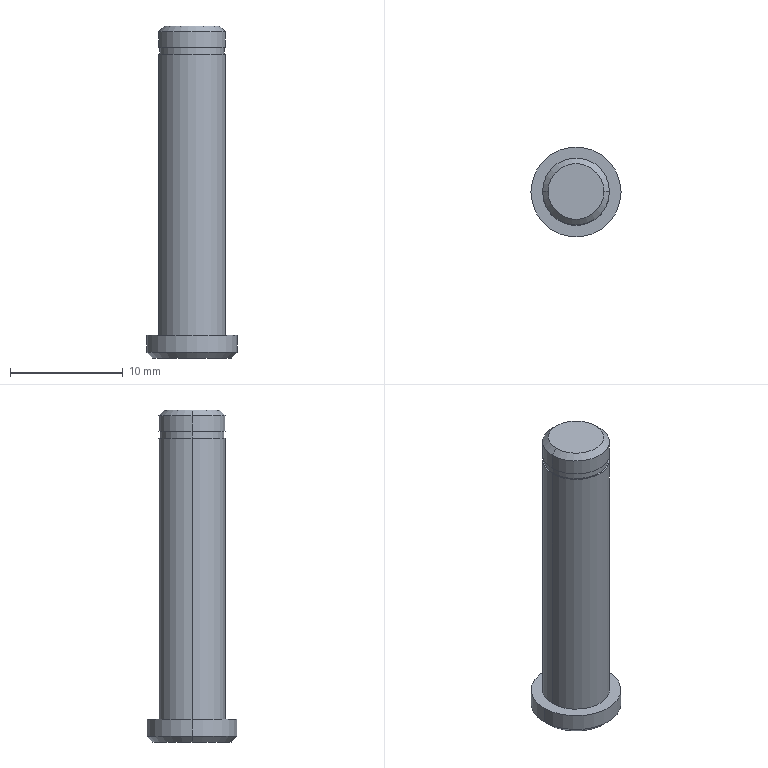Part | SolidWorks | features ICE 3, Chamfer 1, Extrusion 1 | 1 solid | 17 faces | box 8 x 8 x 29.5 mm | volume 858.581 mm3 | cylinder 8 | plane 5 | cone 4 | commonest cylinder face diameters 5.95 x4 5.7 x2 8 x2
STEP:
#1=CARTESIAN_POINT('',(2.475,0.,29.5));
#2=VERTEX_POINT('',#1);
#3=CARTESIAN_POINT('',(-2.475,0.,29.5));
#4=VERTEX_POINT('',#3);
#5=CARTESIAN_POINT('',(0.,0.,29.5));
#6=DIRECTION('',(0.,0.,1.));
#7=DIRECTION('',(1.,0.,0.));
#8=AXIS2_PLACEMENT_3D('',#5,#6,#7);
#9=CIRCLE('',#8,2.475);
#10=EDGE_CURVE('',#2,#4,#9,.T.);
#11=ORIENTED_EDGE('',*,*,#10,.F.);
#12=CARTESIAN_POINT('',(2.975,0.,29.));
#13=VERTEX_POINT('',#12);
#14=CARTESIAN_POINT('',(2.475,0.,29.5));
#15=DIRECTION('',(0.7071,0.,-0.7071));
#16=VECTOR('',#15,1000.);
#17=LINE('',#14,#16);
#18=EDGE_CURVE('',#2,#13,#17,.T.);
#19=ORIENTED_EDGE('',*,*,#18,.T.);
#20=CARTESIAN_POINT('',(-2.975,0.,29.));
#21=VERTEX_POINT('',#20);
#22=CARTESIAN_POINT('',(0.,0.,29.));
#23=DIRECTION('',(0.,0.,-1.));
#24=DIRECTION('',(1.,0.,0.));
#25=AXIS2_PLACEMENT_3D('',#22,#23,#24);
#26=CIRCLE('',#25,2.975);
#27=EDGE_CURVE('',#21,#13,#26,.T.);
#28=ORIENTED_EDGE('',*,*,#27,.F.);
#29=CARTESIAN_POINT('',(-2.475,0.,29.5));
#30=DIRECTION('',(-0.7071,0.,-0.7071));
#31=VECTOR('',#30,1000.);
#32=LINE('',#29,#31);
#33=EDGE_CURVE('',#4,#21,#32,.T.);
#34=ORIENTED_EDGE('',*,*,#33,.F.);
#35=EDGE_LOOP('',(#11,#19,#28,#34));
#36=FACE_OUTER_BOUND('',#35,.T.);
#37=CARTESIAN_POINT('',(0.,0.,29.5));
#38=DIRECTION('',(0.,0.,-1.));
#39=DIRECTION('',(-1.,0.,0.));
#40=AXIS2_PLACEMENT_3D('',#37,#38,#39);
#41=CONICAL_SURFACE('',#40,2.475,0.7854);
#42=ADVANCED_FACE('',(#36),#41,.T.);
#43=CARTESIAN_POINT('',(-3.5,0.,0.));
#44=VERTEX_POINT('',#43);
#45=CARTESIAN_POINT('',(3.5,0.,0.));
#46=VERTEX_POINT('',#45);
#47=CARTESIAN_POINT('',(0.,0.,0.));
#48=DIRECTION('',(0.,0.,-1.));
#49=DIRECTION('',(1.,0.,0.));
#50=AXIS2_PLACEMENT_3D('',#47,#48,#49);
#51=CIRCLE('',#50,3.5);
#52=EDGE_CURVE('',#44,#46,#51,.T.);
#53=ORIENTED_EDGE('',*,*,#52,.F.);
#54=CARTESIAN_POINT('',(-4.,0.,0.5));
#55=VERTEX_POINT('',#54);
#56=CARTESIAN_POINT('',(-4.,0.,0.5));
#57=DIRECTION('',(-0.7071,0.,0.7071));
#58=VECTOR('',#57,1000.);
#59=LINE('',#56,#58);
#60=EDGE_CURVE('',#44,#55,#59,.T.);
#61=ORIENTED_EDGE('',*,*,#60,.T.);
#62=CARTESIAN_POINT('',(4.,0.,0.5));
#63=VERTEX_POINT('',#62);
#64=CARTESIAN_POINT('',(0.,0.,0.5));
#65=DIRECTION('',(0.,0.,1.));
#66=DIRECTION('',(1.,0.,0.));
#67=AXIS2_PLACEMENT_3D('',#64,#65,#66);
#68=CIRCLE('',#67,4.);
#69=EDGE_CURVE('',#63,#55,#68,.T.);
#70=ORIENTED_EDGE('',*,*,#69,.F.);
#71=CARTESIAN_POINT('',(4.,0.,0.5));
#72=DIRECTION('',(0.7071,0.,0.7071));
#73=VECTOR('',#72,1000.);
#74=LINE('',#71,#73);
#75=EDGE_CURVE('',#46,#63,#74,.T.);
#76=ORIENTED_EDGE('',*,*,#75,.F.);
#77=EDGE_LOOP('',(#53,#61,#70,#76));
#78=FACE_OUTER_BOUND('',#77,.T.);
#79=CARTESIAN_POINT('',(0.,0.,0.5));
#80=DIRECTION('',(0.,0.,1.));
#81=DIRECTION('',(1.,0.,0.));
#82=AXIS2_PLACEMENT_3D('',#79,#80,#81);
#83=CONICAL_SURFACE('',#82,4.,0.7854);
#84=ADVANCED_FACE('',(#78),#83,.T.);
#85=ORIENTED_EDGE('',*,*,#27,.T.);
#86=CARTESIAN_POINT('',(2.975,0.,27.6));
#87=VERTEX_POINT('',#86);
#88=CARTESIAN_POINT('',(2.975,0.,29.5));
#89=DIRECTION('',(0.,0.,-1.));
#90=VECTOR('',#89,1000.);
#91=LINE('',#88,#90);
#92=EDGE_CURVE('',#13,#87,#91,.T.);
#93=ORIENTED_EDGE('',*,*,#92,.T.);
#94=CARTESIAN_POINT('',(-2.975,0.,27.6));
#95=VERTEX_POINT('',#94);
#96=CARTESIAN_POINT('',(0.,0.,27.6));
#97=DIRECTION('',(0.,0.,1.));
#98=DIRECTION('',(1.,0.,0.));
#99=AXIS2_PLACEMENT_3D('',#96,#97,#98);
#100=CIRCLE('',#99,2.975);
#101=EDGE_CURVE('',#87,#95,#100,.T.);
#102=ORIENTED_EDGE('',*,*,#101,.T.);
#103=CARTESIAN_POINT('',(-2.975,0.,29.5));
#104=DIRECTION('',(0.,0.,-1.));
#105=VECTOR('',#104,1000.);
#106=LINE('',#103,#105);
#107=EDGE_CURVE('',#21,#95,#106,.T.);
#108=ORIENTED_EDGE('',*,*,#107,.F.);
#109=EDGE_LOOP('',(#85,#93,#102,#108));
#110=FACE_OUTER_BOUND('',#109,.T.);
#111=CARTESIAN_POINT('',(0.,0.,29.5));
#112=DIRECTION('',(0.,0.,-1.));
#113=DIRECTION('',(-1.,0.,0.));
#114=AXIS2_PLACEMENT_3D('',#111,#112,#113);
#115=CYLINDRICAL_SURFACE('',#114,2.975);
#116=ADVANCED_FACE('',(#110),#115,.T.);
#117=CARTESIAN_POINT('',(2.85,0.,27.6));
#118=VERTEX_POINT('',#117);
#119=CARTESIAN_POINT('',(-2.85,0.,27.6));
#120=VERTEX_POINT('',#119);
#121=CARTESIAN_POINT('',(0.,0.,27.6));
#122=DIRECTION('',(0.,0.,1.));
#123=DIRECTION('',(1.,0.,0.));
#124=AXIS2_PLACEMENT_3D('',#121,#122,#123);
#125=CIRCLE('',#124,2.85);
#126=EDGE_CURVE('',#118,#120,#125,.T.);
#127=ORIENTED_EDGE('',*,*,#126,.F.);
#128=CARTESIAN_POINT('',(2.85,0.,27.));
#129=VERTEX_POINT('',#128);
#130=CARTESIAN_POINT('',(2.85,0.,27.6));
#131=DIRECTION('',(0.,0.,-1.));
#132=VECTOR('',#131,1000.);
#133=LINE('',#130,#132);
#134=EDGE_CURVE('',#118,#129,#133,.T.);
#135=ORIENTED_EDGE('',*,*,#134,.T.);
#136=CARTESIAN_POINT('',(-2.85,0.,27.));
#137=VERTEX_POINT('',#136);
#138=CARTESIAN_POINT('',(0.,0.,27.));
#139=DIRECTION('',(0.,0.,1.));
#140=DIRECTION('',(1.,0.,0.));
#141=AXIS2_PLACEMENT_3D('',#138,#139,#140);
#142=CIRCLE('',#141,2.85);
#143=EDGE_CURVE('',#129,#137,#142,.T.);
#144=ORIENTED_EDGE('',*,*,#143,.T.);
#145=CARTESIAN_POINT('',(-2.85,0.,27.6));
#146=DIRECTION('',(0.,0.,-1.));
#147=VECTOR('',#146,1000.);
#148=LINE('',#145,#147);
#149=EDGE_CURVE('',#120,#137,#148,.T.);
#150=ORIENTED_EDGE('',*,*,#149,.F.);
#151=EDGE_LOOP('',(#127,#135,#144,#150));
#152=FACE_OUTER_BOUND('',#151,.T.);
#153=CARTESIAN_POINT('',(0.,0.,27.6));
#154=DIRECTION('',(0.,0.,-1.));
#155=DIRECTION('',(-1.,0.,0.));
#156=AXIS2_PLACEMENT_3D('',#153,#154,#155);
#157=CYLINDRICAL_SURFACE('',#156,2.85);
#158=ADVANCED_FACE('',(#152),#157,.T.);
#159=CARTESIAN_POINT('',(2.975,0.,27.));
#160=VERTEX_POINT('',#159);
#161=CARTESIAN_POINT('',(-2.975,0.,27.));
#162=VERTEX_POINT('',#161);
#163=CARTESIAN_POINT('',(0.,0.,27.));
#164=DIRECTION('',(0.,0.,1.));
#165=DIRECTION('',(1.,0.,0.));
#166=AXIS2_PLACEMENT_3D('',#163,#164,#165);
#167=CIRCLE('',#166,2.975);
#168=EDGE_CURVE('',#160,#162,#167,.T.);
#169=ORIENTED_EDGE('',*,*,#168,.F.);
#170=CARTESIAN_POINT('',(2.975,0.,2.));
#171=VERTEX_POINT('',#170);
#172=CARTESIAN_POINT('',(2.975,0.,27.));
#173=DIRECTION('',(0.,0.,-1.));
#174=VECTOR('',#173,1000.);
#175=LINE('',#172,#174);
#176=EDGE_CURVE('',#160,#171,#175,.T.);
#177=ORIENTED_EDGE('',*,*,#176,.T.);
#178=CARTESIAN_POINT('',(-2.975,0.,2.));
#179=VERTEX_POINT('',#178);
#180=CARTESIAN_POINT('',(0.,0.,2.));
#181=DIRECTION('',(0.,0.,1.));
#182=DIRECTION('',(1.,0.,0.));
#183=AXIS2_PLACEMENT_3D('',#180,#181,#182);
#184=CIRCLE('',#183,2.975);
#185=EDGE_CURVE('',#171,#179,#184,.T.);
#186=ORIENTED_EDGE('',*,*,#185,.T.);
#187=CARTESIAN_POINT('',(-2.975,0.,27.));
#188=DIRECTION('',(0.,0.,-1.));
#189=VECTOR('',#188,1000.);
#190=LINE('',#187,#189);
#191=EDGE_CURVE('',#162,#179,#190,.T.);
#192=ORIENTED_EDGE('',*,*,#191,.F.);
#193=EDGE_LOOP('',(#169,#177,#186,#192));
#194=FACE_OUTER_BOUND('',#193,.T.);
#195=CARTESIAN_POINT('',(0.,0.,27.));
#196=DIRECTION('',(0.,0.,-1.));
#197=DIRECTION('',(-1.,0.,0.));
#198=AXIS2_PLACEMENT_3D('',#195,#196,#197);
#199=CYLINDRICAL_SURFACE('',#198,2.975);
#200=ADVANCED_FACE('',(#194),#199,.T.);
#201=CARTESIAN_POINT('',(4.,0.,2.));
#202=VERTEX_POINT('',#201);
#203=CARTESIAN_POINT('',(-4.,0.,2.));
#204=VERTEX_POINT('',#203);
#205=CARTESIAN_POINT('',(0.,0.,2.));
#206=DIRECTION('',(0.,0.,1.));
#207=DIRECTION('',(1.,0.,0.));
#208=AXIS2_PLACEMENT_3D('',#205,#206,#207);
#209=CIRCLE('',#208,4.);
#210=EDGE_CURVE('',#202,#204,#209,.T.);
#211=ORIENTED_EDGE('',*,*,#210,.F.);
#212=CARTESIAN_POINT('',(4.,0.,2.));
#213=DIRECTION('',(0.,0.,-1.));
#214=VECTOR('',#213,1000.);
#215=LINE('',#212,#214);
#216=EDGE_CURVE('',#202,#63,#215,.T.);
#217=ORIENTED_EDGE('',*,*,#216,.T.);
#218=ORIENTED_EDGE('',*,*,#69,.T.);
#219=CARTESIAN_POINT('',(-4.,0.,2.));
#220=DIRECTION('',(0.,0.,-1.));
#221=VECTOR('',#220,1000.);
#222=LINE('',#219,#221);
#223=EDGE_CURVE('',#204,#55,#222,.T.);
#224=ORIENTED_EDGE('',*,*,#223,.F.);
#225=EDGE_LOOP('',(#211,#217,#218,#224));
#226=FACE_OUTER_BOUND('',#225,.T.);
#227=CARTESIAN_POINT('',(0.,0.,2.));
#228=DIRECTION('',(0.,0.,-1.));
#229=DIRECTION('',(-1.,0.,0.));
#230=AXIS2_PLACEMENT_3D('',#227,#228,#229);
#231=CYLINDRICAL_SURFACE('',#230,4.);
#232=ADVANCED_FACE('',(#226),#231,.T.);
#233=ORIENTED_EDGE('',*,*,#216,.F.);
#234=CARTESIAN_POINT('',(0.,0.,2.));
#235=DIRECTION('',(0.,0.,1.));
#236=DIRECTION('',(1.,0.,0.));
#237=AXIS2_PLACEMENT_3D('',#234,#235,#236);
#238=CIRCLE('',#237,4.);
#239=EDGE_CURVE('',#204,#202,#238,.T.);
#240=ORIENTED_EDGE('',*,*,#239,.F.);
#241=ORIENTED_EDGE('',*,*,#223,.T.);
#242=CARTESIAN_POINT('',(0.,0.,0.5));
#243=DIRECTION('',(0.,0.,1.));
#244=DIRECTION('',(1.,0.,0.));
#245=AXIS2_PLACEMENT_3D('',#242,#243,#244);
#246=CIRCLE('',#245,4.);
#247=EDGE_CURVE('',#55,#63,#246,.T.);
#248=ORIENTED_EDGE('',*,*,#247,.T.);
#249=EDGE_LOOP('',(#233,#240,#241,#248));
#250=FACE_OUTER_BOUND('',#249,.T.);
#251=CARTESIAN_POINT('',(0.,0.,2.));
#252=DIRECTION('',(0.,0.,-1.));
#253=DIRECTION('',(-1.,0.,0.));
#254=AXIS2_PLACEMENT_3D('',#251,#252,#253);
#255=CYLINDRICAL_SURFACE('',#254,4.);
#256=ADVANCED_FACE('',(#250),#255,.T.);
#257=CARTESIAN_POINT('',(0.,0.,2.));
#258=DIRECTION('',(0.,0.,1.));
#259=DIRECTION('',(1.,0.,0.));
#260=AXIS2_PLACEMENT_3D('',#257,#258,#259);
#261=CIRCLE('',#260,2.975);
#262=EDGE_CURVE('',#179,#171,#261,.T.);
#263=ORIENTED_EDGE('',*,*,#262,.F.);
#264=ORIENTED_EDGE('',*,*,#185,.F.);
#265=EDGE_LOOP('',(#263,#264));
#266=FACE_BOUND('',#265,.T.);
#267=ORIENTED_EDGE('',*,*,#239,.T.);
#268=ORIENTED_EDGE('',*,*,#210,.T.);
#269=EDGE_LOOP('',(#267,#268));
#270=FACE_OUTER_BOUND('',#269,.T.);
#271=CARTESIAN_POINT('',(0.,0.,2.));
#272=DIRECTION('',(0.,0.,1.));
#273=DIRECTION('',(1.,0.,0.));
#274=AXIS2_PLACEMENT_3D('',#271,#272,#273);
#275=PLANE('',#274);
#276=ADVANCED_FACE('',(#266,#270),#275,.T.);
#277=CARTESIAN_POINT('',(0.,0.,0.));
#278=DIRECTION('',(0.,0.,-1.));
#279=DIRECTION('',(1.,0.,0.));
#280=AXIS2_PLACEMENT_3D('',#277,#278,#279);
#281=CIRCLE('',#280,3.5);
#282=EDGE_CURVE('',#46,#44,#281,.T.);
#283=ORIENTED_EDGE('',*,*,#282,.T.);
#284=ORIENTED_EDGE('',*,*,#52,.T.);
#285=EDGE_LOOP('',(#283,#284));
#286=FACE_OUTER_BOUND('',#285,.T.);
#287=CARTESIAN_POINT('',(0.,0.,0.));
#288=DIRECTION('',(0.,0.,1.));
#289=DIRECTION('',(1.,0.,0.));
#290=AXIS2_PLACEMENT_3D('',#287,#288,#289);
#291=PLANE('',#290);
#292=ADVANCED_FACE('',(#286),#291,.F.);
#293=ORIENTED_EDGE('',*,*,#176,.F.);
#294=CARTESIAN_POINT('',(0.,0.,27.));
#295=DIRECTION('',(0.,0.,1.));
#296=DIRECTION('',(1.,0.,0.));
#297=AXIS2_PLACEMENT_3D('',#294,#295,#296);
#298=CIRCLE('',#297,2.975);
#299=EDGE_CURVE('',#162,#160,#298,.T.);
#300=ORIENTED_EDGE('',*,*,#299,.F.);
#301=ORIENTED_EDGE('',*,*,#191,.T.);
#302=ORIENTED_EDGE('',*,*,#262,.T.);
#303=EDGE_LOOP('',(#293,#300,#301,#302));
#304=FACE_OUTER_BOUND('',#303,.T.);
#305=CARTESIAN_POINT('',(0.,0.,27.));
#306=DIRECTION('',(0.,0.,-1.));
#307=DIRECTION('',(-1.,0.,0.));
#308=AXIS2_PLACEMENT_3D('',#305,#306,#307);
#309=CYLINDRICAL_SURFACE('',#308,2.975);
#310=ADVANCED_FACE('',(#304),#309,.T.);
#311=CARTESIAN_POINT('',(0.,0.,27.));
#312=DIRECTION('',(0.,0.,1.));
#313=DIRECTION('',(1.,0.,0.));
#314=AXIS2_PLACEMENT_3D('',#311,#312,#313);
#315=CIRCLE('',#314,2.85);
#316=EDGE_CURVE('',#137,#129,#315,.T.);
#317=ORIENTED_EDGE('',*,*,#316,.F.);
#318=ORIENTED_EDGE('',*,*,#143,.F.);
#319=EDGE_LOOP('',(#317,#318));
#320=FACE_BOUND('',#319,.T.);
#321=ORIENTED_EDGE('',*,*,#299,.T.);
#322=ORIENTED_EDGE('',*,*,#168,.T.);
#323=EDGE_LOOP('',(#321,#322));
#324=FACE_OUTER_BOUND('',#323,.T.);
#325=CARTESIAN_POINT('',(0.,0.,27.));
#326=DIRECTION('',(0.,0.,1.));
#327=DIRECTION('',(1.,0.,0.));
#328=AXIS2_PLACEMENT_3D('',#325,#326,#327);
#329=PLANE('',#328);
#330=ADVANCED_FACE('',(#320,#324),#329,.T.);
#331=ORIENTED_EDGE('',*,*,#134,.F.);
#332=CARTESIAN_POINT('',(0.,0.,27.6));
#333=DIRECTION('',(0.,0.,1.));
#334=DIRECTION('',(1.,0.,0.));
#335=AXIS2_PLACEMENT_3D('',#332,#333,#334);
#336=CIRCLE('',#335,2.85);
#337=EDGE_CURVE('',#120,#118,#336,.T.);
#338=ORIENTED_EDGE('',*,*,#337,.F.);
#339=ORIENTED_EDGE('',*,*,#149,.T.);
#340=ORIENTED_EDGE('',*,*,#316,.T.);
#341=EDGE_LOOP('',(#331,#338,#339,#340));
#342=FACE_OUTER_BOUND('',#341,.T.);
#343=CARTESIAN_POINT('',(0.,0.,27.6));
#344=DIRECTION('',(0.,0.,-1.));
#345=DIRECTION('',(-1.,0.,0.));
#346=AXIS2_PLACEMENT_3D('',#343,#344,#345);
#347=CYLINDRICAL_SURFACE('',#346,2.85);
#348=ADVANCED_FACE('',(#342),#347,.T.);
#349=ORIENTED_EDGE('',*,*,#92,.F.);
#350=CARTESIAN_POINT('',(0.,0.,29.));
#351=DIRECTION('',(0.,0.,-1.));
#352=DIRECTION('',(1.,0.,0.));
#353=AXIS2_PLACEMENT_3D('',#350,#351,#352);
#354=CIRCLE('',#353,2.975);
#355=EDGE_CURVE('',#13,#21,#354,.T.);
#356=ORIENTED_EDGE('',*,*,#355,.T.);
#357=ORIENTED_EDGE('',*,*,#107,.T.);
#358=CARTESIAN_POINT('',(0.,0.,27.6));
#359=DIRECTION('',(0.,0.,1.));
#360=DIRECTION('',(1.,0.,0.));
#361=AXIS2_PLACEMENT_3D('',#358,#359,#360);
#362=CIRCLE('',#361,2.975);
#363=EDGE_CURVE('',#95,#87,#362,.T.);
#364=ORIENTED_EDGE('',*,*,#363,.T.);
#365=EDGE_LOOP('',(#349,#356,#357,#364));
#366=FACE_OUTER_BOUND('',#365,.T.);
#367=CARTESIAN_POINT('',(0.,0.,29.5));
#368=DIRECTION('',(0.,0.,-1.));
#369=DIRECTION('',(-1.,0.,0.));
#370=AXIS2_PLACEMENT_3D('',#367,#368,#369);
#371=CYLINDRICAL_SURFACE('',#370,2.975);
#372=ADVANCED_FACE('',(#366),#371,.T.);
#373=CARTESIAN_POINT('',(0.,0.,29.5));
#374=DIRECTION('',(0.,0.,1.));
#375=DIRECTION('',(1.,0.,0.));
#376=AXIS2_PLACEMENT_3D('',#373,#374,#375);
#377=CIRCLE('',#376,2.475);
#378=EDGE_CURVE('',#4,#2,#377,.T.);
#379=ORIENTED_EDGE('',*,*,#378,.T.);
#380=ORIENTED_EDGE('',*,*,#10,.T.);
#381=EDGE_LOOP('',(#379,#380));
#382=FACE_OUTER_BOUND('',#381,.T.);
#383=CARTESIAN_POINT('',(0.,0.,29.5));
#384=DIRECTION('',(0.,0.,1.));
#385=DIRECTION('',(1.,0.,0.));
#386=AXIS2_PLACEMENT_3D('',#383,#384,#385);
#387=PLANE('',#386);
#388=ADVANCED_FACE('',(#382),#387,.T.);
#389=ORIENTED_EDGE('',*,*,#337,.T.);
#390=ORIENTED_EDGE('',*,*,#126,.T.);
#391=EDGE_LOOP('',(#389,#390));
#392=FACE_BOUND('',#391,.T.);
#393=ORIENTED_EDGE('',*,*,#363,.F.);
#394=ORIENTED_EDGE('',*,*,#101,.F.);
#395=EDGE_LOOP('',(#393,#394));
#396=FACE_OUTER_BOUND('',#395,.T.);
#397=CARTESIAN_POINT('',(0.,0.,27.6));
#398=DIRECTION('',(0.,0.,1.));
#399=DIRECTION('',(1.,0.,0.));
#400=AXIS2_PLACEMENT_3D('',#397,#398,#399);
#401=PLANE('',#400);
#402=ADVANCED_FACE('',(#392,#396),#401,.F.);
#403=ORIENTED_EDGE('',*,*,#60,.F.);
#404=ORIENTED_EDGE('',*,*,#282,.F.);
#405=ORIENTED_EDGE('',*,*,#75,.T.);
#406=ORIENTED_EDGE('',*,*,#247,.F.);
#407=EDGE_LOOP('',(#403,#404,#405,#406));
#408=FACE_OUTER_BOUND('',#407,.T.);
#409=CARTESIAN_POINT('',(0.,0.,0.5));
#410=DIRECTION('',(0.,0.,1.));
#411=DIRECTION('',(1.,0.,0.));
#412=AXIS2_PLACEMENT_3D('',#409,#410,#411);
#413=CONICAL_SURFACE('',#412,4.,0.7854);
#414=ADVANCED_FACE('',(#408),#413,.T.);
#415=ORIENTED_EDGE('',*,*,#18,.F.);
#416=ORIENTED_EDGE('',*,*,#378,.F.);
#417=ORIENTED_EDGE('',*,*,#33,.T.);
#418=ORIENTED_EDGE('',*,*,#355,.F.);
#419=EDGE_LOOP('',(#415,#416,#417,#418));
#420=FACE_OUTER_BOUND('',#419,.T.);
#421=CARTESIAN_POINT('',(0.,0.,29.5));
#422=DIRECTION('',(0.,0.,-1.));
#423=DIRECTION('',(-1.,0.,0.));
#424=AXIS2_PLACEMENT_3D('',#421,#422,#423);
#425=CONICAL_SURFACE('',#424,2.475,0.7854);
#426=ADVANCED_FACE('',(#420),#425,.T.);
#427=CLOSED_SHELL('',(#42,#84,#116,#158,#200,#232,#256,#276,#292,#310,#330,#348,#372,#388,#402,#414,#426));
#428=MANIFOLD_SOLID_BREP('',#427);
#429=CARTESIAN_POINT('',(0.,0.,0.));
#430=DIRECTION('',(0.,0.,1.));
#431=DIRECTION('',(1.,0.,0.));
#432=AXIS2_PLACEMENT_3D('',#429,#430,#431);
#433=(LENGTH_UNIT()NAMED_UNIT(*)SI_UNIT(.MILLI.,.METRE.));
#434=UNCERTAINTY_MEASURE_WITH_UNIT(LENGTH_MEASURE(0.00001),#433,'','');
#435=(NAMED_UNIT(*)PLANE_ANGLE_UNIT()SI_UNIT($,.RADIAN.));
#436=(NAMED_UNIT(*)SI_UNIT($,.STERADIAN.)SOLID_ANGLE_UNIT());
#437=(GEOMETRIC_REPRESENTATION_CONTEXT(3)GLOBAL_UNCERTAINTY_ASSIGNED_CONTEXT((#434))GLOBAL_UNIT_ASSIGNED_CONTEXT((#433,#435,#436))REPRESENTATION_CONTEXT('',''));
#438=ADVANCED_BREP_SHAPE_REPRESENTATION('',(#428,#432),#437);